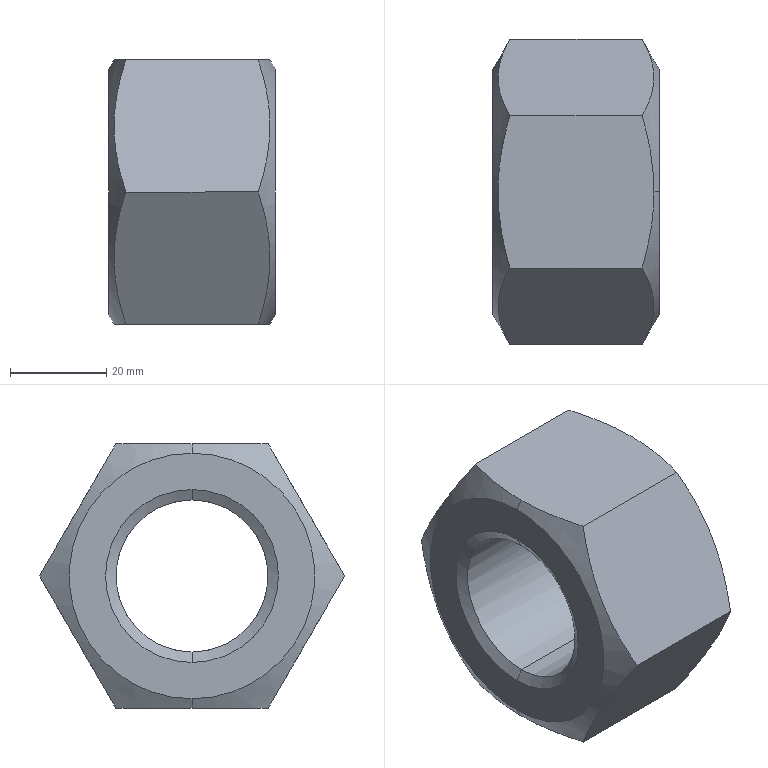Part | STEP file | 1 solid | 18 faces | box 34.7 x 63.509 x 55 mm | volume 62007 mm3 | cone 8 | plane 8 | cylinder 2 | commonest cylinder face diameters 31.67 x2